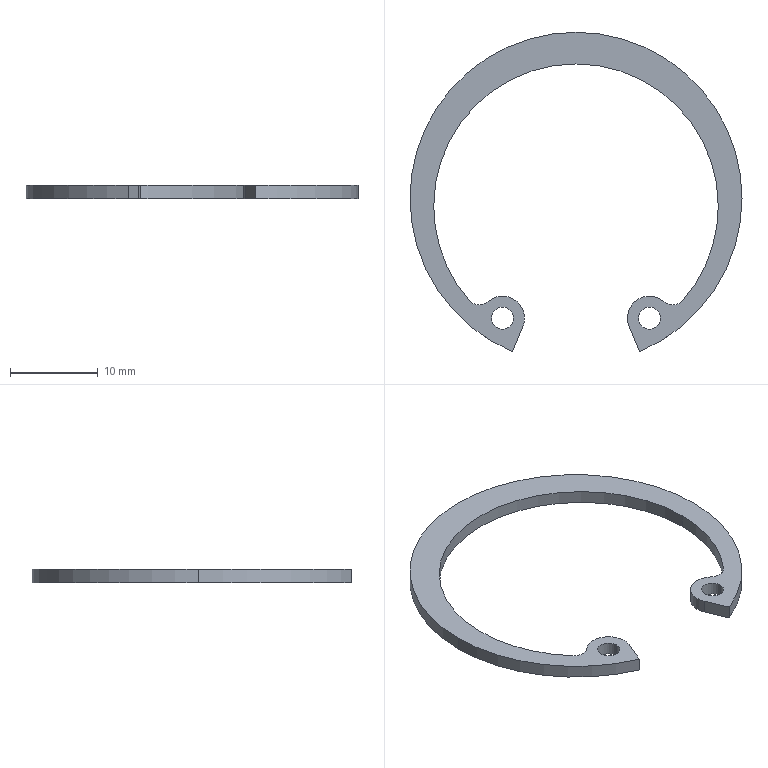Part | SolidWorks | features Extrusion 1 | 1 solid | 19 faces | box 37.8 x 36.361 x 1.5 mm | volume 438.212 mm3 | cylinder 15 | plane 4 | commonest cylinder face diameters 2.5 x4 5 x3 32.4 x3 37.8 x3 3 x2
STEP:
#1=CARTESIAN_POINT('',(-9.607,-13.644,-1.5));
#2=VERTEX_POINT('',#1);
#3=CARTESIAN_POINT('',(-7.107,-13.644,-1.5));
#4=VERTEX_POINT('',#3);
#5=CARTESIAN_POINT('',(-8.357,-13.644,-1.5));
#6=DIRECTION('',(0.,0.,1.));
#7=DIRECTION('',(1.,0.,0.));
#8=AXIS2_PLACEMENT_3D('',#5,#6,#7);
#9=CIRCLE('',#8,1.25);
#10=EDGE_CURVE('',#2,#4,#9,.T.);
#11=ORIENTED_EDGE('',*,*,#10,.F.);
#12=CARTESIAN_POINT('',(-9.607,-13.644,0.));
#13=VERTEX_POINT('',#12);
#14=CARTESIAN_POINT('',(-9.607,-13.644,-1.5));
#15=DIRECTION('',(0.,0.,1.));
#16=VECTOR('',#15,1000.);
#17=LINE('',#14,#16);
#18=EDGE_CURVE('',#2,#13,#17,.T.);
#19=ORIENTED_EDGE('',*,*,#18,.T.);
#20=CARTESIAN_POINT('',(-7.107,-13.644,0.));
#21=VERTEX_POINT('',#20);
#22=CARTESIAN_POINT('',(-8.357,-13.644,0.));
#23=DIRECTION('',(0.,0.,1.));
#24=DIRECTION('',(1.,0.,0.));
#25=AXIS2_PLACEMENT_3D('',#22,#23,#24);
#26=CIRCLE('',#25,1.25);
#27=EDGE_CURVE('',#13,#21,#26,.T.);
#28=ORIENTED_EDGE('',*,*,#27,.T.);
#29=CARTESIAN_POINT('',(-7.107,-13.644,-1.5));
#30=DIRECTION('',(0.,0.,1.));
#31=VECTOR('',#30,1000.);
#32=LINE('',#29,#31);
#33=EDGE_CURVE('',#4,#21,#32,.T.);
#34=ORIENTED_EDGE('',*,*,#33,.F.);
#35=EDGE_LOOP('',(#11,#19,#28,#34));
#36=FACE_OUTER_BOUND('',#35,.T.);
#37=CARTESIAN_POINT('',(-8.357,-13.644,-1.5));
#38=DIRECTION('',(0.,0.,1.));
#39=DIRECTION('',(1.,0.,0.));
#40=AXIS2_PLACEMENT_3D('',#37,#38,#39);
#41=CYLINDRICAL_SURFACE('',#40,1.25);
#42=ADVANCED_FACE('',(#36),#41,.F.);
#43=CARTESIAN_POINT('',(7.107,-13.644,-1.5));
#44=VERTEX_POINT('',#43);
#45=CARTESIAN_POINT('',(9.607,-13.644,-1.5));
#46=VERTEX_POINT('',#45);
#47=CARTESIAN_POINT('',(8.357,-13.644,-1.5));
#48=DIRECTION('',(0.,0.,1.));
#49=DIRECTION('',(-1.,0.,0.));
#50=AXIS2_PLACEMENT_3D('',#47,#48,#49);
#51=CIRCLE('',#50,1.25);
#52=EDGE_CURVE('',#44,#46,#51,.T.);
#53=ORIENTED_EDGE('',*,*,#52,.F.);
#54=CARTESIAN_POINT('',(7.107,-13.644,0.));
#55=VERTEX_POINT('',#54);
#56=CARTESIAN_POINT('',(7.107,-13.644,-1.5));
#57=DIRECTION('',(0.,0.,1.));
#58=VECTOR('',#57,1000.);
#59=LINE('',#56,#58);
#60=EDGE_CURVE('',#44,#55,#59,.T.);
#61=ORIENTED_EDGE('',*,*,#60,.T.);
#62=CARTESIAN_POINT('',(9.607,-13.644,0.));
#63=VERTEX_POINT('',#62);
#64=CARTESIAN_POINT('',(8.357,-13.644,0.));
#65=DIRECTION('',(0.,0.,1.));
#66=DIRECTION('',(-1.,0.,0.));
#67=AXIS2_PLACEMENT_3D('',#64,#65,#66);
#68=CIRCLE('',#67,1.25);
#69=EDGE_CURVE('',#55,#63,#68,.T.);
#70=ORIENTED_EDGE('',*,*,#69,.T.);
#71=CARTESIAN_POINT('',(9.607,-13.644,-1.5));
#72=DIRECTION('',(0.,0.,1.));
#73=VECTOR('',#72,1000.);
#74=LINE('',#71,#73);
#75=EDGE_CURVE('',#46,#63,#74,.T.);
#76=ORIENTED_EDGE('',*,*,#75,.F.);
#77=EDGE_LOOP('',(#53,#61,#70,#76));
#78=FACE_OUTER_BOUND('',#77,.T.);
#79=CARTESIAN_POINT('',(8.357,-13.644,-1.5));
#80=DIRECTION('',(0.,0.,1.));
#81=DIRECTION('',(1.,0.,0.));
#82=AXIS2_PLACEMENT_3D('',#79,#80,#81);
#83=CYLINDRICAL_SURFACE('',#82,1.25);
#84=ADVANCED_FACE('',(#78),#83,.F.);
#85=CARTESIAN_POINT('',(-6.048,-14.601,-1.5));
#86=VERTEX_POINT('',#85);
#87=CARTESIAN_POINT('',(-5.857,-13.644,-1.5));
#88=VERTEX_POINT('',#87);
#89=CARTESIAN_POINT('',(-8.357,-13.644,-1.5));
#90=DIRECTION('',(0.,0.,1.));
#91=DIRECTION('',(1.,0.,0.));
#92=AXIS2_PLACEMENT_3D('',#89,#90,#91);
#93=CIRCLE('',#92,2.5);
#94=EDGE_CURVE('',#86,#88,#93,.T.);
#95=ORIENTED_EDGE('',*,*,#94,.T.);
#96=CARTESIAN_POINT('',(-5.857,-13.644,0.));
#97=VERTEX_POINT('',#96);
#98=CARTESIAN_POINT('',(-5.857,-13.644,-1.5));
#99=DIRECTION('',(0.,0.,1.));
#100=VECTOR('',#99,1000.);
#101=LINE('',#98,#100);
#102=EDGE_CURVE('',#88,#97,#101,.T.);
#103=ORIENTED_EDGE('',*,*,#102,.T.);
#104=CARTESIAN_POINT('',(-6.048,-14.601,0.));
#105=VERTEX_POINT('',#104);
#106=CARTESIAN_POINT('',(-8.357,-13.644,0.));
#107=DIRECTION('',(0.,0.,1.));
#108=DIRECTION('',(1.,0.,0.));
#109=AXIS2_PLACEMENT_3D('',#106,#107,#108);
#110=CIRCLE('',#109,2.5);
#111=EDGE_CURVE('',#105,#97,#110,.T.);
#112=ORIENTED_EDGE('',*,*,#111,.F.);
#113=CARTESIAN_POINT('',(-6.048,-14.601,-1.5));
#114=DIRECTION('',(0.,0.,1.));
#115=VECTOR('',#114,1000.);
#116=LINE('',#113,#115);
#117=EDGE_CURVE('',#86,#105,#116,.T.);
#118=ORIENTED_EDGE('',*,*,#117,.F.);
#119=EDGE_LOOP('',(#95,#103,#112,#118));
#120=FACE_OUTER_BOUND('',#119,.T.);
#121=CARTESIAN_POINT('',(-8.357,-13.644,-1.5));
#122=DIRECTION('',(0.,0.,1.));
#123=DIRECTION('',(1.,0.,0.));
#124=AXIS2_PLACEMENT_3D('',#121,#122,#123);
#125=CYLINDRICAL_SURFACE('',#124,2.5);
#126=ADVANCED_FACE('',(#120),#125,.T.);
#127=CARTESIAN_POINT('',(-12.128,-11.64,-1.5));
#128=VERTEX_POINT('',#127);
#129=CARTESIAN_POINT('',(-16.2,-0.9,-1.5));
#130=VERTEX_POINT('',#129);
#131=CARTESIAN_POINT('',(0.,-0.9,-1.5));
#132=DIRECTION('',(0.,0.,-1.));
#133=DIRECTION('',(1.,0.,0.));
#134=AXIS2_PLACEMENT_3D('',#131,#132,#133);
#135=CIRCLE('',#134,16.2);
#136=EDGE_CURVE('',#128,#130,#135,.T.);
#137=ORIENTED_EDGE('',*,*,#136,.T.);
#138=CARTESIAN_POINT('',(-16.2,-0.9,0.));
#139=VERTEX_POINT('',#138);
#140=CARTESIAN_POINT('',(-16.2,-0.9,-1.5));
#141=DIRECTION('',(0.,0.,1.));
#142=VECTOR('',#141,1000.);
#143=LINE('',#140,#142);
#144=EDGE_CURVE('',#130,#139,#143,.T.);
#145=ORIENTED_EDGE('',*,*,#144,.T.);
#146=CARTESIAN_POINT('',(-12.128,-11.64,0.));
#147=VERTEX_POINT('',#146);
#148=CARTESIAN_POINT('',(0.,-0.9,0.));
#149=DIRECTION('',(0.,0.,-1.));
#150=DIRECTION('',(1.,0.,0.));
#151=AXIS2_PLACEMENT_3D('',#148,#149,#150);
#152=CIRCLE('',#151,16.2);
#153=EDGE_CURVE('',#147,#139,#152,.T.);
#154=ORIENTED_EDGE('',*,*,#153,.F.);
#155=CARTESIAN_POINT('',(-12.128,-11.64,-1.5));
#156=DIRECTION('',(0.,0.,1.));
#157=VECTOR('',#156,1000.);
#158=LINE('',#155,#157);
#159=EDGE_CURVE('',#128,#147,#158,.T.);
#160=ORIENTED_EDGE('',*,*,#159,.F.);
#161=EDGE_LOOP('',(#137,#145,#154,#160));
#162=FACE_OUTER_BOUND('',#161,.T.);
#163=CARTESIAN_POINT('',(0.,-0.9,-1.5));
#164=DIRECTION('',(0.,0.,1.));
#165=DIRECTION('',(1.,0.,0.));
#166=AXIS2_PLACEMENT_3D('',#163,#164,#165);
#167=CYLINDRICAL_SURFACE('',#166,16.2);
#168=ADVANCED_FACE('',(#162),#167,.F.);
#169=ORIENTED_EDGE('',*,*,#144,.F.);
#170=CARTESIAN_POINT('',(16.2,-0.9,-1.5));
#171=VERTEX_POINT('',#170);
#172=CARTESIAN_POINT('',(0.,-0.9,-1.5));
#173=DIRECTION('',(0.,0.,-1.));
#174=DIRECTION('',(1.,0.,0.));
#175=AXIS2_PLACEMENT_3D('',#172,#173,#174);
#176=CIRCLE('',#175,16.2);
#177=EDGE_CURVE('',#130,#171,#176,.T.);
#178=ORIENTED_EDGE('',*,*,#177,.T.);
#179=CARTESIAN_POINT('',(16.2,-0.9,0.));
#180=VERTEX_POINT('',#179);
#181=CARTESIAN_POINT('',(16.2,-0.9,-1.5));
#182=DIRECTION('',(0.,0.,1.));
#183=VECTOR('',#182,1000.);
#184=LINE('',#181,#183);
#185=EDGE_CURVE('',#171,#180,#184,.T.);
#186=ORIENTED_EDGE('',*,*,#185,.T.);
#187=CARTESIAN_POINT('',(0.,-0.9,0.));
#188=DIRECTION('',(0.,0.,-1.));
#189=DIRECTION('',(1.,0.,0.));
#190=AXIS2_PLACEMENT_3D('',#187,#188,#189);
#191=CIRCLE('',#190,16.2);
#192=EDGE_CURVE('',#139,#180,#191,.T.);
#193=ORIENTED_EDGE('',*,*,#192,.F.);
#194=EDGE_LOOP('',(#169,#178,#186,#193));
#195=FACE_OUTER_BOUND('',#194,.T.);
#196=CARTESIAN_POINT('',(0.,-0.9,-1.5));
#197=DIRECTION('',(0.,0.,1.));
#198=DIRECTION('',(1.,0.,0.));
#199=AXIS2_PLACEMENT_3D('',#196,#197,#198);
#200=CYLINDRICAL_SURFACE('',#199,16.2);
#201=ADVANCED_FACE('',(#195),#200,.F.);
#202=CARTESIAN_POINT('',(18.9,0.,-1.5));
#203=VERTEX_POINT('',#202);
#204=CARTESIAN_POINT('',(-18.9,0.,-1.5));
#205=VERTEX_POINT('',#204);
#206=CARTESIAN_POINT('',(0.,0.,-1.5));
#207=DIRECTION('',(0.,0.,1.));
#208=DIRECTION('',(1.,0.,0.));
#209=AXIS2_PLACEMENT_3D('',#206,#207,#208);
#210=CIRCLE('',#209,18.9);
#211=EDGE_CURVE('',#203,#205,#210,.T.);
#212=ORIENTED_EDGE('',*,*,#211,.T.);
#213=CARTESIAN_POINT('',(-18.9,0.,0.));
#214=VERTEX_POINT('',#213);
#215=CARTESIAN_POINT('',(-18.9,0.,-1.5));
#216=DIRECTION('',(0.,0.,1.));
#217=VECTOR('',#216,1000.);
#218=LINE('',#215,#217);
#219=EDGE_CURVE('',#205,#214,#218,.T.);
#220=ORIENTED_EDGE('',*,*,#219,.T.);
#221=CARTESIAN_POINT('',(18.9,0.,0.));
#222=VERTEX_POINT('',#221);
#223=CARTESIAN_POINT('',(0.,0.,0.));
#224=DIRECTION('',(0.,0.,1.));
#225=DIRECTION('',(1.,0.,0.));
#226=AXIS2_PLACEMENT_3D('',#223,#224,#225);
#227=CIRCLE('',#226,18.9);
#228=EDGE_CURVE('',#222,#214,#227,.T.);
#229=ORIENTED_EDGE('',*,*,#228,.F.);
#230=CARTESIAN_POINT('',(18.9,0.,-1.5));
#231=DIRECTION('',(0.,0.,1.));
#232=VECTOR('',#231,1000.);
#233=LINE('',#230,#232);
#234=EDGE_CURVE('',#203,#222,#233,.T.);
#235=ORIENTED_EDGE('',*,*,#234,.F.);
#236=EDGE_LOOP('',(#212,#220,#229,#235));
#237=FACE_OUTER_BOUND('',#236,.T.);
#238=CARTESIAN_POINT('',(0.,0.,-1.5));
#239=DIRECTION('',(0.,0.,1.));
#240=DIRECTION('',(1.,0.,0.));
#241=AXIS2_PLACEMENT_3D('',#238,#239,#240);
#242=CYLINDRICAL_SURFACE('',#241,18.9);
#243=ADVANCED_FACE('',(#237),#242,.T.);
#244=CARTESIAN_POINT('',(7.233,-17.461,-1.5));
#245=VERTEX_POINT('',#244);
#246=CARTESIAN_POINT('',(0.,0.,-1.5));
#247=DIRECTION('',(0.,0.,1.));
#248=DIRECTION('',(1.,0.,0.));
#249=AXIS2_PLACEMENT_3D('',#246,#247,#248);
#250=CIRCLE('',#249,18.9);
#251=EDGE_CURVE('',#245,#203,#250,.T.);
#252=ORIENTED_EDGE('',*,*,#251,.T.);
#253=ORIENTED_EDGE('',*,*,#234,.T.);
#254=CARTESIAN_POINT('',(7.233,-17.461,0.));
#255=VERTEX_POINT('',#254);
#256=CARTESIAN_POINT('',(0.,0.,0.));
#257=DIRECTION('',(0.,0.,1.));
#258=DIRECTION('',(1.,0.,0.));
#259=AXIS2_PLACEMENT_3D('',#256,#257,#258);
#260=CIRCLE('',#259,18.9);
#261=EDGE_CURVE('',#255,#222,#260,.T.);
#262=ORIENTED_EDGE('',*,*,#261,.F.);
#263=CARTESIAN_POINT('',(7.233,-17.461,-1.5));
#264=DIRECTION('',(0.,0.,1.));
#265=VECTOR('',#264,1000.);
#266=LINE('',#263,#265);
#267=EDGE_CURVE('',#245,#255,#266,.T.);
#268=ORIENTED_EDGE('',*,*,#267,.F.);
#269=EDGE_LOOP('',(#252,#253,#262,#268));
#270=FACE_OUTER_BOUND('',#269,.T.);
#271=CARTESIAN_POINT('',(0.,0.,-1.5));
#272=DIRECTION('',(0.,0.,1.));
#273=DIRECTION('',(1.,0.,0.));
#274=AXIS2_PLACEMENT_3D('',#271,#272,#273);
#275=CYLINDRICAL_SURFACE('',#274,18.9);
#276=ADVANCED_FACE('',(#270),#275,.T.);
#277=ORIENTED_EDGE('',*,*,#219,.F.);
#278=CARTESIAN_POINT('',(-7.233,-17.461,-1.5));
#279=VERTEX_POINT('',#278);
#280=CARTESIAN_POINT('',(0.,0.,-1.5));
#281=DIRECTION('',(0.,0.,1.));
#282=DIRECTION('',(1.,0.,0.));
#283=AXIS2_PLACEMENT_3D('',#280,#281,#282);
#284=CIRCLE('',#283,18.9);
#285=EDGE_CURVE('',#205,#279,#284,.T.);
#286=ORIENTED_EDGE('',*,*,#285,.T.);
#287=CARTESIAN_POINT('',(-7.233,-17.461,0.));
#288=VERTEX_POINT('',#287);
#289=CARTESIAN_POINT('',(-7.233,-17.461,-1.5));
#290=DIRECTION('',(0.,0.,1.));
#291=VECTOR('',#290,1000.);
#292=LINE('',#289,#291);
#293=EDGE_CURVE('',#279,#288,#292,.T.);
#294=ORIENTED_EDGE('',*,*,#293,.T.);
#295=CARTESIAN_POINT('',(0.,0.,0.));
#296=DIRECTION('',(0.,0.,1.));
#297=DIRECTION('',(1.,0.,0.));
#298=AXIS2_PLACEMENT_3D('',#295,#296,#297);
#299=CIRCLE('',#298,18.9);
#300=EDGE_CURVE('',#214,#288,#299,.T.);
#301=ORIENTED_EDGE('',*,*,#300,.F.);
#302=EDGE_LOOP('',(#277,#286,#294,#301));
#303=FACE_OUTER_BOUND('',#302,.T.);
#304=CARTESIAN_POINT('',(0.,0.,-1.5));
#305=DIRECTION('',(0.,0.,1.));
#306=DIRECTION('',(1.,0.,0.));
#307=AXIS2_PLACEMENT_3D('',#304,#305,#306);
#308=CYLINDRICAL_SURFACE('',#307,18.9);
#309=ADVANCED_FACE('',(#303),#308,.T.);
#310=CARTESIAN_POINT('',(6.048,-14.601,0.));
#311=VERTEX_POINT('',#310);
#312=CARTESIAN_POINT('',(6.048,-14.601,0.));
#313=DIRECTION('',(0.3827,-0.9239,0.));
#314=VECTOR('',#313,1000.);
#315=LINE('',#312,#314);
#316=EDGE_CURVE('',#311,#255,#315,.T.);
#317=ORIENTED_EDGE('',*,*,#316,.F.);
#318=CARTESIAN_POINT('',(6.048,-14.601,-1.5));
#319=VERTEX_POINT('',#318);
#320=CARTESIAN_POINT('',(6.048,-14.601,-1.5));
#321=DIRECTION('',(0.,0.,1.));
#322=VECTOR('',#321,1000.);
#323=LINE('',#320,#322);
#324=EDGE_CURVE('',#319,#311,#323,.T.);
#325=ORIENTED_EDGE('',*,*,#324,.F.);
#326=CARTESIAN_POINT('',(6.048,-14.601,-1.5));
#327=DIRECTION('',(0.3827,-0.9239,0.));
#328=VECTOR('',#327,1000.);
#329=LINE('',#326,#328);
#330=EDGE_CURVE('',#319,#245,#329,.T.);
#331=ORIENTED_EDGE('',*,*,#330,.T.);
#332=ORIENTED_EDGE('',*,*,#267,.T.);
#333=EDGE_LOOP('',(#317,#325,#331,#332));
#334=FACE_OUTER_BOUND('',#333,.T.);
#335=CARTESIAN_POINT('',(6.048,-14.601,-1.5));
#336=DIRECTION('',(-0.9239,-0.3827,0.));
#337=DIRECTION('',(0.3827,-0.9239,0.));
#338=AXIS2_PLACEMENT_3D('',#335,#336,#337);
#339=PLANE('',#338);
#340=ADVANCED_FACE('',(#334),#339,.T.);
#341=CARTESIAN_POINT('',(10.012,-11.77,0.));
#342=VERTEX_POINT('',#341);
#343=CARTESIAN_POINT('',(8.357,-13.644,0.));
#344=DIRECTION('',(0.,0.,1.));
#345=DIRECTION('',(-1.,0.,0.));
#346=AXIS2_PLACEMENT_3D('',#343,#344,#345);
#347=CIRCLE('',#346,2.5);
#348=EDGE_CURVE('',#342,#311,#347,.T.);
#349=ORIENTED_EDGE('',*,*,#348,.F.);
#350=CARTESIAN_POINT('',(10.012,-11.77,-1.5));
#351=VERTEX_POINT('',#350);
#352=CARTESIAN_POINT('',(10.012,-11.77,-1.5));
#353=DIRECTION('',(0.,0.,1.));
#354=VECTOR('',#353,1000.);
#355=LINE('',#352,#354);
#356=EDGE_CURVE('',#351,#342,#355,.T.);
#357=ORIENTED_EDGE('',*,*,#356,.F.);
#358=CARTESIAN_POINT('',(8.357,-13.644,-1.5));
#359=DIRECTION('',(0.,0.,1.));
#360=DIRECTION('',(-1.,0.,0.));
#361=AXIS2_PLACEMENT_3D('',#358,#359,#360);
#362=CIRCLE('',#361,2.5);
#363=EDGE_CURVE('',#351,#319,#362,.T.);
#364=ORIENTED_EDGE('',*,*,#363,.T.);
#365=ORIENTED_EDGE('',*,*,#324,.T.);
#366=EDGE_LOOP('',(#349,#357,#364,#365));
#367=FACE_OUTER_BOUND('',#366,.T.);
#368=CARTESIAN_POINT('',(8.357,-13.644,-1.5));
#369=DIRECTION('',(0.,0.,1.));
#370=DIRECTION('',(1.,0.,0.));
#371=AXIS2_PLACEMENT_3D('',#368,#369,#370);
#372=CYLINDRICAL_SURFACE('',#371,2.5);
#373=ADVANCED_FACE('',(#367),#372,.T.);
#374=CARTESIAN_POINT('',(12.128,-11.64,0.));
#375=VERTEX_POINT('',#374);
#376=CARTESIAN_POINT('',(11.005,-10.646,0.));
#377=DIRECTION('',(0.,0.,-1.));
#378=DIRECTION('',(-1.,0.,0.));
#379=AXIS2_PLACEMENT_3D('',#376,#377,#378);
#380=CIRCLE('',#379,1.5);
#381=EDGE_CURVE('',#375,#342,#380,.T.);
#382=ORIENTED_EDGE('',*,*,#381,.F.);
#383=CARTESIAN_POINT('',(12.128,-11.64,-1.5));
#384=VERTEX_POINT('',#383);
#385=CARTESIAN_POINT('',(12.128,-11.64,-1.5));
#386=DIRECTION('',(0.,0.,1.));
#387=VECTOR('',#386,1000.);
#388=LINE('',#385,#387);
#389=EDGE_CURVE('',#384,#375,#388,.T.);
#390=ORIENTED_EDGE('',*,*,#389,.F.);
#391=CARTESIAN_POINT('',(11.005,-10.646,-1.5));
#392=DIRECTION('',(0.,0.,-1.));
#393=DIRECTION('',(-1.,0.,0.));
#394=AXIS2_PLACEMENT_3D('',#391,#392,#393);
#395=CIRCLE('',#394,1.5);
#396=EDGE_CURVE('',#384,#351,#395,.T.);
#397=ORIENTED_EDGE('',*,*,#396,.T.);
#398=ORIENTED_EDGE('',*,*,#356,.T.);
#399=EDGE_LOOP('',(#382,#390,#397,#398));
#400=FACE_OUTER_BOUND('',#399,.T.);
#401=CARTESIAN_POINT('',(11.005,-10.646,-1.5));
#402=DIRECTION('',(0.,0.,1.));
#403=DIRECTION('',(1.,0.,0.));
#404=AXIS2_PLACEMENT_3D('',#401,#402,#403);
#405=CYLINDRICAL_SURFACE('',#404,1.5);
#406=ADVANCED_FACE('',(#400),#405,.F.);
#407=ORIENTED_EDGE('',*,*,#185,.F.);
#408=CARTESIAN_POINT('',(0.,-0.9,-1.5));
#409=DIRECTION('',(0.,0.,-1.));
#410=DIRECTION('',(1.,0.,0.));
#411=AXIS2_PLACEMENT_3D('',#408,#409,#410);
#412=CIRCLE('',#411,16.2);
#413=EDGE_CURVE('',#171,#384,#412,.T.);
#414=ORIENTED_EDGE('',*,*,#413,.T.);
#415=ORIENTED_EDGE('',*,*,#389,.T.);
#416=CARTESIAN_POINT('',(0.,-0.9,0.));
#417=DIRECTION('',(0.,0.,-1.));
#418=DIRECTION('',(1.,0.,0.));
#419=AXIS2_PLACEMENT_3D('',#416,#417,#418);
#420=CIRCLE('',#419,16.2);
#421=EDGE_CURVE('',#180,#375,#420,.T.);
#422=ORIENTED_EDGE('',*,*,#421,.F.);
#423=EDGE_LOOP('',(#407,#414,#415,#422));
#424=FACE_OUTER_BOUND('',#423,.T.);
#425=CARTESIAN_POINT('',(0.,-0.9,-1.5));
#426=DIRECTION('',(0.,0.,1.));
#427=DIRECTION('',(1.,0.,0.));
#428=AXIS2_PLACEMENT_3D('',#425,#426,#427);
#429=CYLINDRICAL_SURFACE('',#428,16.2);
#430=ADVANCED_FACE('',(#424),#429,.F.);
#431=CARTESIAN_POINT('',(-10.012,-11.77,0.));
#432=VERTEX_POINT('',#431);
#433=CARTESIAN_POINT('',(-11.005,-10.646,0.));
#434=DIRECTION('',(0.,0.,-1.));
#435=DIRECTION('',(1.,0.,0.));
#436=AXIS2_PLACEMENT_3D('',#433,#434,#435);
#437=CIRCLE('',#436,1.5);
#438=EDGE_CURVE('',#432,#147,#437,.T.);
#439=ORIENTED_EDGE('',*,*,#438,.F.);
#440=CARTESIAN_POINT('',(-10.012,-11.77,-1.5));
#441=VERTEX_POINT('',#440);
#442=CARTESIAN_POINT('',(-10.012,-11.77,-1.5));
#443=DIRECTION('',(0.,0.,1.));
#444=VECTOR('',#443,1000.);
#445=LINE('',#442,#444);
#446=EDGE_CURVE('',#441,#432,#445,.T.);
#447=ORIENTED_EDGE('',*,*,#446,.F.);
#448=CARTESIAN_POINT('',(-11.005,-10.646,-1.5));
#449=DIRECTION('',(0.,0.,-1.));
#450=DIRECTION('',(1.,0.,0.));
#451=AXIS2_PLACEMENT_3D('',#448,#449,#450);
#452=CIRCLE('',#451,1.5);
#453=EDGE_CURVE('',#441,#128,#452,.T.);
#454=ORIENTED_EDGE('',*,*,#453,.T.);
#455=ORIENTED_EDGE('',*,*,#159,.T.);
#456=EDGE_LOOP('',(#439,#447,#454,#455));
#457=FACE_OUTER_BOUND('',#456,.T.);
#458=CARTESIAN_POINT('',(-11.005,-10.646,-1.5));
#459=DIRECTION('',(0.,0.,1.));
#460=DIRECTION('',(1.,0.,0.));
#461=AXIS2_PLACEMENT_3D('',#458,#459,#460);
#462=CYLINDRICAL_SURFACE('',#461,1.5);
#463=ADVANCED_FACE('',(#457),#462,.F.);
#464=ORIENTED_EDGE('',*,*,#102,.F.);
#465=CARTESIAN_POINT('',(-8.357,-13.644,-1.5));
#466=DIRECTION('',(0.,0.,1.));
#467=DIRECTION('',(1.,0.,0.));
#468=AXIS2_PLACEMENT_3D('',#465,#466,#467);
#469=CIRCLE('',#468,2.5);
#470=EDGE_CURVE('',#88,#441,#469,.T.);
#471=ORIENTED_EDGE('',*,*,#470,.T.);
#472=ORIENTED_EDGE('',*,*,#446,.T.);
#473=CARTESIAN_POINT('',(-8.357,-13.644,0.));
#474=DIRECTION('',(0.,0.,1.));
#475=DIRECTION('',(1.,0.,0.));
#476=AXIS2_PLACEMENT_3D('',#473,#474,#475);
#477=CIRCLE('',#476,2.5);
#478=EDGE_CURVE('',#97,#432,#477,.T.);
#479=ORIENTED_EDGE('',*,*,#478,.F.);
#480=EDGE_LOOP('',(#464,#471,#472,#479));
#481=FACE_OUTER_BOUND('',#480,.T.);
#482=CARTESIAN_POINT('',(-8.357,-13.644,-1.5));
#483=DIRECTION('',(0.,0.,1.));
#484=DIRECTION('',(1.,0.,0.));
#485=AXIS2_PLACEMENT_3D('',#482,#483,#484);
#486=CYLINDRICAL_SURFACE('',#485,2.5);
#487=ADVANCED_FACE('',(#481),#486,.T.);
#488=CARTESIAN_POINT('',(-6.048,-14.601,0.));
#489=DIRECTION('',(0.3827,0.9239,0.));
#490=VECTOR('',#489,1000.);
#491=LINE('',#488,#490);
#492=EDGE_CURVE('',#288,#105,#491,.T.);
#493=ORIENTED_EDGE('',*,*,#492,.F.);
#494=ORIENTED_EDGE('',*,*,#293,.F.);
#495=CARTESIAN_POINT('',(-6.048,-14.601,-1.5));
#496=DIRECTION('',(0.3827,0.9239,0.));
#497=VECTOR('',#496,1000.);
#498=LINE('',#495,#497);
#499=EDGE_CURVE('',#279,#86,#498,.T.);
#500=ORIENTED_EDGE('',*,*,#499,.T.);
#501=ORIENTED_EDGE('',*,*,#117,.T.);
#502=EDGE_LOOP('',(#493,#494,#500,#501));
#503=FACE_OUTER_BOUND('',#502,.T.);
#504=CARTESIAN_POINT('',(-6.048,-14.601,-1.5));
#505=DIRECTION('',(0.9239,-0.3827,0.));
#506=DIRECTION('',(0.3827,0.9239,0.));
#507=AXIS2_PLACEMENT_3D('',#504,#505,#506);
#508=PLANE('',#507);
#509=ADVANCED_FACE('',(#503),#508,.T.);
#510=CARTESIAN_POINT('',(-8.357,-13.644,-1.5));
#511=DIRECTION('',(0.,0.,1.));
#512=DIRECTION('',(1.,0.,0.));
#513=AXIS2_PLACEMENT_3D('',#510,#511,#512);
#514=CIRCLE('',#513,1.25);
#515=EDGE_CURVE('',#4,#2,#514,.T.);
#516=ORIENTED_EDGE('',*,*,#515,.T.);
#517=ORIENTED_EDGE('',*,*,#10,.T.);
#518=EDGE_LOOP('',(#516,#517));
#519=FACE_BOUND('',#518,.T.);
#520=CARTESIAN_POINT('',(8.357,-13.644,-1.5));
#521=DIRECTION('',(0.,0.,1.));
#522=DIRECTION('',(-1.,0.,0.));
#523=AXIS2_PLACEMENT_3D('',#520,#521,#522);
#524=CIRCLE('',#523,1.25);
#525=EDGE_CURVE('',#46,#44,#524,.T.);
#526=ORIENTED_EDGE('',*,*,#525,.T.);
#527=ORIENTED_EDGE('',*,*,#52,.T.);
#528=EDGE_LOOP('',(#526,#527));
#529=FACE_BOUND('',#528,.T.);
#530=ORIENTED_EDGE('',*,*,#251,.F.);
#531=ORIENTED_EDGE('',*,*,#330,.F.);
#532=ORIENTED_EDGE('',*,*,#363,.F.);
#533=ORIENTED_EDGE('',*,*,#396,.F.);
#534=ORIENTED_EDGE('',*,*,#413,.F.);
#535=ORIENTED_EDGE('',*,*,#177,.F.);
#536=ORIENTED_EDGE('',*,*,#136,.F.);
#537=ORIENTED_EDGE('',*,*,#453,.F.);
#538=ORIENTED_EDGE('',*,*,#470,.F.);
#539=ORIENTED_EDGE('',*,*,#94,.F.);
#540=ORIENTED_EDGE('',*,*,#499,.F.);
#541=ORIENTED_EDGE('',*,*,#285,.F.);
#542=ORIENTED_EDGE('',*,*,#211,.F.);
#543=EDGE_LOOP('',(#530,#531,#532,#533,#534,#535,#536,#537,#538,#539,#540,#541,#542));
#544=FACE_OUTER_BOUND('',#543,.T.);
#545=CARTESIAN_POINT('',(0.,0.,-1.5));
#546=DIRECTION('',(0.,0.,1.));
#547=DIRECTION('',(1.,0.,0.));
#548=AXIS2_PLACEMENT_3D('',#545,#546,#547);
#549=PLANE('',#548);
#550=ADVANCED_FACE('',(#519,#529,#544),#549,.F.);
#551=CARTESIAN_POINT('',(-8.357,-13.644,0.));
#552=DIRECTION('',(0.,0.,1.));
#553=DIRECTION('',(1.,0.,0.));
#554=AXIS2_PLACEMENT_3D('',#551,#552,#553);
#555=CIRCLE('',#554,1.25);
#556=EDGE_CURVE('',#21,#13,#555,.T.);
#557=ORIENTED_EDGE('',*,*,#556,.F.);
#558=ORIENTED_EDGE('',*,*,#27,.F.);
#559=EDGE_LOOP('',(#557,#558));
#560=FACE_BOUND('',#559,.T.);
#561=CARTESIAN_POINT('',(8.357,-13.644,0.));
#562=DIRECTION('',(0.,0.,1.));
#563=DIRECTION('',(-1.,0.,0.));
#564=AXIS2_PLACEMENT_3D('',#561,#562,#563);
#565=CIRCLE('',#564,1.25);
#566=EDGE_CURVE('',#63,#55,#565,.T.);
#567=ORIENTED_EDGE('',*,*,#566,.F.);
#568=ORIENTED_EDGE('',*,*,#69,.F.);
#569=EDGE_LOOP('',(#567,#568));
#570=FACE_BOUND('',#569,.T.);
#571=ORIENTED_EDGE('',*,*,#261,.T.);
#572=ORIENTED_EDGE('',*,*,#228,.T.);
#573=ORIENTED_EDGE('',*,*,#300,.T.);
#574=ORIENTED_EDGE('',*,*,#492,.T.);
#575=ORIENTED_EDGE('',*,*,#111,.T.);
#576=ORIENTED_EDGE('',*,*,#478,.T.);
#577=ORIENTED_EDGE('',*,*,#438,.T.);
#578=ORIENTED_EDGE('',*,*,#153,.T.);
#579=ORIENTED_EDGE('',*,*,#192,.T.);
#580=ORIENTED_EDGE('',*,*,#421,.T.);
#581=ORIENTED_EDGE('',*,*,#381,.T.);
#582=ORIENTED_EDGE('',*,*,#348,.T.);
#583=ORIENTED_EDGE('',*,*,#316,.T.);
#584=EDGE_LOOP('',(#571,#572,#573,#574,#575,#576,#577,#578,#579,#580,#581,#582,#583));
#585=FACE_OUTER_BOUND('',#584,.T.);
#586=CARTESIAN_POINT('',(0.,0.,0.));
#587=DIRECTION('',(0.,0.,1.));
#588=DIRECTION('',(1.,0.,0.));
#589=AXIS2_PLACEMENT_3D('',#586,#587,#588);
#590=PLANE('',#589);
#591=ADVANCED_FACE('',(#560,#570,#585),#590,.T.);
#592=ORIENTED_EDGE('',*,*,#60,.F.);
#593=ORIENTED_EDGE('',*,*,#525,.F.);
#594=ORIENTED_EDGE('',*,*,#75,.T.);
#595=ORIENTED_EDGE('',*,*,#566,.T.);
#596=EDGE_LOOP('',(#592,#593,#594,#595));
#597=FACE_OUTER_BOUND('',#596,.T.);
#598=CARTESIAN_POINT('',(8.357,-13.644,-1.5));
#599=DIRECTION('',(0.,0.,1.));
#600=DIRECTION('',(1.,0.,0.));
#601=AXIS2_PLACEMENT_3D('',#598,#599,#600);
#602=CYLINDRICAL_SURFACE('',#601,1.25);
#603=ADVANCED_FACE('',(#597),#602,.F.);
#604=ORIENTED_EDGE('',*,*,#18,.F.);
#605=ORIENTED_EDGE('',*,*,#515,.F.);
#606=ORIENTED_EDGE('',*,*,#33,.T.);
#607=ORIENTED_EDGE('',*,*,#556,.T.);
#608=EDGE_LOOP('',(#604,#605,#606,#607));
#609=FACE_OUTER_BOUND('',#608,.T.);
#610=CARTESIAN_POINT('',(-8.357,-13.644,-1.5));
#611=DIRECTION('',(0.,0.,1.));
#612=DIRECTION('',(1.,0.,0.));
#613=AXIS2_PLACEMENT_3D('',#610,#611,#612);
#614=CYLINDRICAL_SURFACE('',#613,1.25);
#615=ADVANCED_FACE('',(#609),#614,.F.);
#616=CLOSED_SHELL('',(#42,#84,#126,#168,#201,#243,#276,#309,#340,#373,#406,#430,#463,#487,#509,#550,#591,#603,#615));
#617=MANIFOLD_SOLID_BREP('',#616);
#618=CARTESIAN_POINT('',(0.,0.,0.));
#619=DIRECTION('',(0.,0.,1.));
#620=DIRECTION('',(1.,0.,0.));
#621=AXIS2_PLACEMENT_3D('',#618,#619,#620);
#622=(LENGTH_UNIT()NAMED_UNIT(*)SI_UNIT(.MILLI.,.METRE.));
#623=UNCERTAINTY_MEASURE_WITH_UNIT(LENGTH_MEASURE(0.00001),#622,'','');
#624=(NAMED_UNIT(*)PLANE_ANGLE_UNIT()SI_UNIT($,.RADIAN.));
#625=(NAMED_UNIT(*)SI_UNIT($,.STERADIAN.)SOLID_ANGLE_UNIT());
#626=(GEOMETRIC_REPRESENTATION_CONTEXT(3)GLOBAL_UNCERTAINTY_ASSIGNED_CONTEXT((#623))GLOBAL_UNIT_ASSIGNED_CONTEXT((#622,#624,#625))REPRESENTATION_CONTEXT('',''));
#627=ADVANCED_BREP_SHAPE_REPRESENTATION('',(#617,#621),#626);